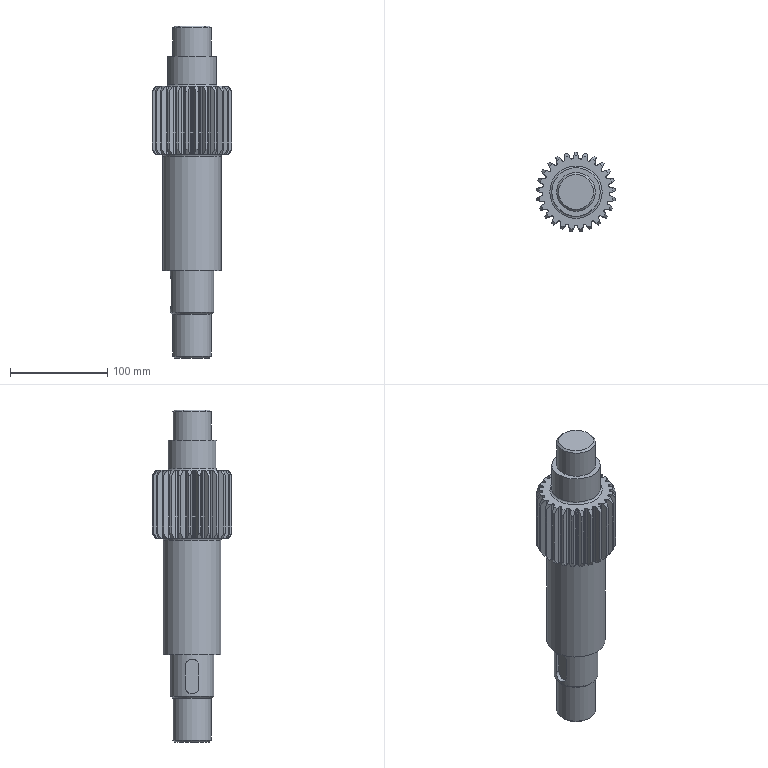Part | NX | features BREP 25, META 25, DATUM_CSYS 5, SKETCH 4, BOSS 3, EXTRUDE 3, CHAMFER 2, BLEND 1, CYLINDER 1, FSET 1, SWP104 1 | 1 solid | 222 faces | box 82.296 x 82.148 x 342.25 mm | volume 879629 mm3 | spline 125 | cone 53 | cylinder 32 | plane 10 | torus 2 | commonest cylinder face diameters 68.625 x25 14 x2 40 x2 45 x1 50 x1 60 x1